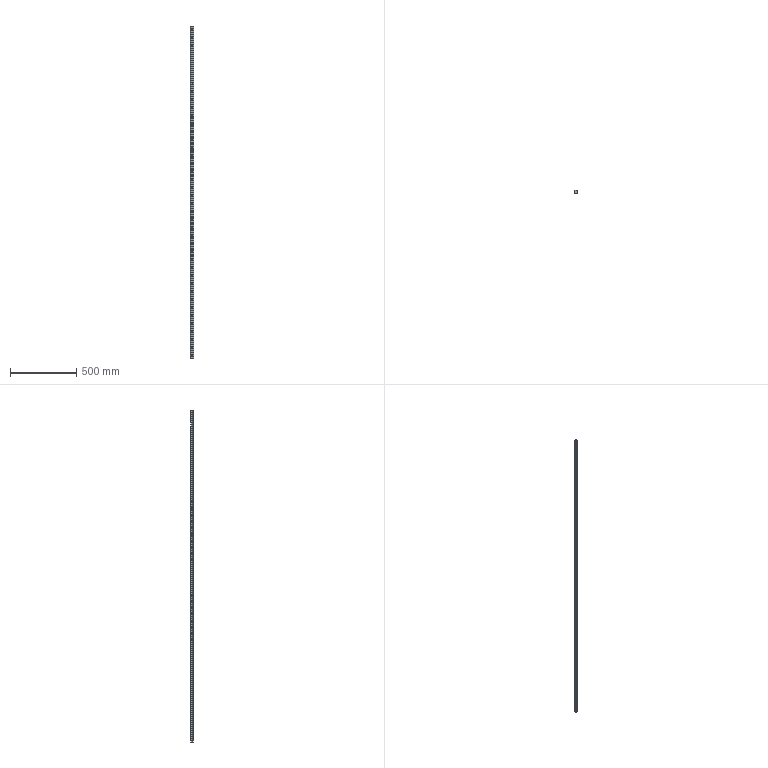Part | SolidWorks | features BaseBody 1, HoleWzd 1, ICE 1, LPattern 1 | 1 solid | 244 faces | box 23 x 22 x 2500 mm | volume 1050284 mm3 | cylinder 172 | plane 72 | commonest cylinder face diameters 11 x84 6.6 x78 7 x6 4.6 x4